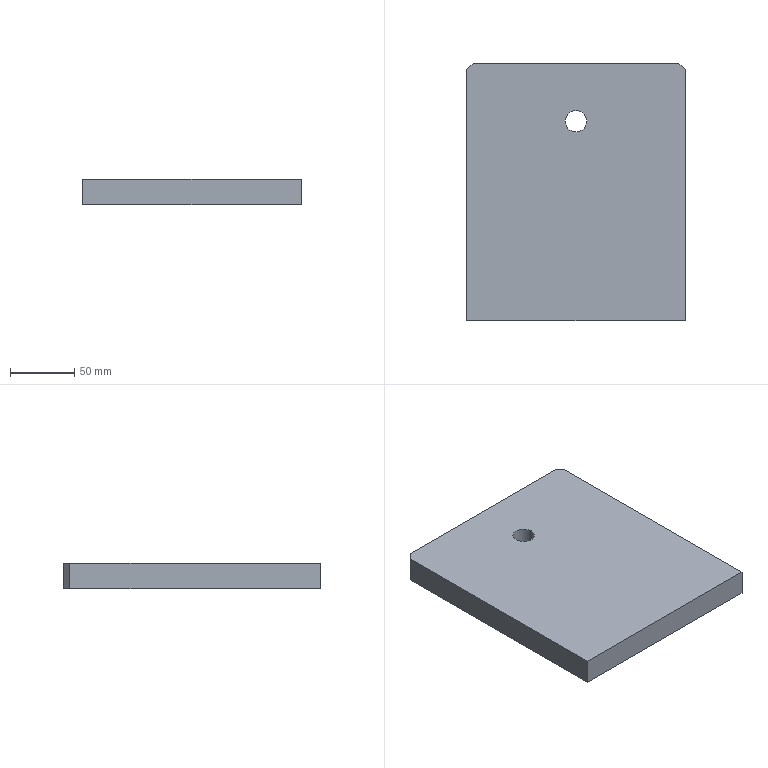Part | SolidWorks | features 3DProfileFeature 1, Extrusion 1, HoleWzd 1 | 1 solid | 10 faces | box 170 x 200 x 20 mm | volume 675136 mm3 | plane 8 | cylinder 2 | commonest cylinder face diameters 16.667 x2
STEP:
#1=CARTESIAN_POINT('',(76.666,155.,0.));
#2=VERTEX_POINT('',#1);
#3=CARTESIAN_POINT('',(93.334,155.,0.));
#4=VERTEX_POINT('',#3);
#5=CARTESIAN_POINT('',(85.,155.,0.));
#6=DIRECTION('',(0.,0.,1.));
#7=DIRECTION('',(1.,0.,0.));
#8=AXIS2_PLACEMENT_3D('',#5,#6,#7);
#9=CIRCLE('',#8,8.334);
#10=EDGE_CURVE('',#2,#4,#9,.T.);
#11=ORIENTED_EDGE('',*,*,#10,.F.);
#12=CARTESIAN_POINT('',(76.666,155.,20.));
#13=VERTEX_POINT('',#12);
#14=CARTESIAN_POINT('',(76.666,155.,20.));
#15=DIRECTION('',(0.,0.,1.));
#16=VECTOR('',#15,1000.);
#17=LINE('',#14,#16);
#18=EDGE_CURVE('',#2,#13,#17,.T.);
#19=ORIENTED_EDGE('',*,*,#18,.T.);
#20=CARTESIAN_POINT('',(93.334,155.,20.));
#21=VERTEX_POINT('',#20);
#22=CARTESIAN_POINT('',(85.,155.,20.));
#23=DIRECTION('',(0.,0.,1.));
#24=DIRECTION('',(1.,0.,0.));
#25=AXIS2_PLACEMENT_3D('',#22,#23,#24);
#26=CIRCLE('',#25,8.334);
#27=EDGE_CURVE('',#13,#21,#26,.T.);
#28=ORIENTED_EDGE('',*,*,#27,.T.);
#29=CARTESIAN_POINT('',(93.334,155.,20.));
#30=DIRECTION('',(0.,0.,1.));
#31=VECTOR('',#30,1000.);
#32=LINE('',#29,#31);
#33=EDGE_CURVE('',#4,#21,#32,.T.);
#34=ORIENTED_EDGE('',*,*,#33,.F.);
#35=EDGE_LOOP('',(#11,#19,#28,#34));
#36=FACE_OUTER_BOUND('',#35,.T.);
#37=CARTESIAN_POINT('',(85.,155.,20.));
#38=DIRECTION('',(0.,0.,1.));
#39=DIRECTION('',(1.,0.,0.));
#40=AXIS2_PLACEMENT_3D('',#37,#38,#39);
#41=CYLINDRICAL_SURFACE('',#40,8.334);
#42=ADVANCED_FACE('',(#36),#41,.F.);
#43=CARTESIAN_POINT('',(0.,195.,0.));
#44=VERTEX_POINT('',#43);
#45=CARTESIAN_POINT('',(0.,0.,0.));
#46=VERTEX_POINT('',#45);
#47=CARTESIAN_POINT('',(0.,0.,0.));
#48=DIRECTION('',(0.,-1.,0.));
#49=VECTOR('',#48,1000.);
#50=LINE('',#47,#49);
#51=EDGE_CURVE('',#44,#46,#50,.T.);
#52=ORIENTED_EDGE('',*,*,#51,.T.);
#53=CARTESIAN_POINT('',(0.,0.,20.));
#54=VERTEX_POINT('',#53);
#55=CARTESIAN_POINT('',(0.,0.,20.));
#56=DIRECTION('',(0.,0.,-1.));
#57=VECTOR('',#56,1000.);
#58=LINE('',#55,#57);
#59=EDGE_CURVE('',#54,#46,#58,.T.);
#60=ORIENTED_EDGE('',*,*,#59,.F.);
#61=CARTESIAN_POINT('',(0.,195.,20.));
#62=VERTEX_POINT('',#61);
#63=CARTESIAN_POINT('',(0.,0.,20.));
#64=DIRECTION('',(0.,-1.,0.));
#65=VECTOR('',#64,1000.);
#66=LINE('',#63,#65);
#67=EDGE_CURVE('',#62,#54,#66,.T.);
#68=ORIENTED_EDGE('',*,*,#67,.F.);
#69=CARTESIAN_POINT('',(0.,195.,20.));
#70=DIRECTION('',(0.,0.,-1.));
#71=VECTOR('',#70,1000.);
#72=LINE('',#69,#71);
#73=EDGE_CURVE('',#62,#44,#72,.T.);
#74=ORIENTED_EDGE('',*,*,#73,.T.);
#75=EDGE_LOOP('',(#52,#60,#68,#74));
#76=FACE_OUTER_BOUND('',#75,.T.);
#77=CARTESIAN_POINT('',(0.,0.,20.));
#78=DIRECTION('',(1.,0.,0.));
#79=DIRECTION('',(0.,0.,-1.));
#80=AXIS2_PLACEMENT_3D('',#77,#78,#79);
#81=PLANE('',#80);
#82=ADVANCED_FACE('',(#76),#81,.F.);
#83=CARTESIAN_POINT('',(170.,0.,0.));
#84=VERTEX_POINT('',#83);
#85=CARTESIAN_POINT('',(0.,0.,0.));
#86=DIRECTION('',(1.,0.,0.));
#87=VECTOR('',#86,1000.);
#88=LINE('',#85,#87);
#89=EDGE_CURVE('',#46,#84,#88,.T.);
#90=ORIENTED_EDGE('',*,*,#89,.T.);
#91=CARTESIAN_POINT('',(170.,0.,20.));
#92=VERTEX_POINT('',#91);
#93=CARTESIAN_POINT('',(170.,0.,20.));
#94=DIRECTION('',(0.,0.,-1.));
#95=VECTOR('',#94,1000.);
#96=LINE('',#93,#95);
#97=EDGE_CURVE('',#92,#84,#96,.T.);
#98=ORIENTED_EDGE('',*,*,#97,.F.);
#99=CARTESIAN_POINT('',(0.,0.,20.));
#100=DIRECTION('',(1.,0.,0.));
#101=VECTOR('',#100,1000.);
#102=LINE('',#99,#101);
#103=EDGE_CURVE('',#54,#92,#102,.T.);
#104=ORIENTED_EDGE('',*,*,#103,.F.);
#105=ORIENTED_EDGE('',*,*,#59,.T.);
#106=EDGE_LOOP('',(#90,#98,#104,#105));
#107=FACE_OUTER_BOUND('',#106,.T.);
#108=CARTESIAN_POINT('',(0.,0.,20.));
#109=DIRECTION('',(0.,1.,0.));
#110=DIRECTION('',(0.,0.,1.));
#111=AXIS2_PLACEMENT_3D('',#108,#109,#110);
#112=PLANE('',#111);
#113=ADVANCED_FACE('',(#107),#112,.F.);
#114=CARTESIAN_POINT('',(170.,195.,0.));
#115=VERTEX_POINT('',#114);
#116=CARTESIAN_POINT('',(170.,0.,0.));
#117=DIRECTION('',(0.,1.,0.));
#118=VECTOR('',#117,1000.);
#119=LINE('',#116,#118);
#120=EDGE_CURVE('',#84,#115,#119,.T.);
#121=ORIENTED_EDGE('',*,*,#120,.T.);
#122=CARTESIAN_POINT('',(170.,195.,20.));
#123=VERTEX_POINT('',#122);
#124=CARTESIAN_POINT('',(170.,195.,20.));
#125=DIRECTION('',(0.,0.,-1.));
#126=VECTOR('',#125,1000.);
#127=LINE('',#124,#126);
#128=EDGE_CURVE('',#123,#115,#127,.T.);
#129=ORIENTED_EDGE('',*,*,#128,.F.);
#130=CARTESIAN_POINT('',(170.,0.,20.));
#131=DIRECTION('',(0.,1.,0.));
#132=VECTOR('',#131,1000.);
#133=LINE('',#130,#132);
#134=EDGE_CURVE('',#92,#123,#133,.T.);
#135=ORIENTED_EDGE('',*,*,#134,.F.);
#136=ORIENTED_EDGE('',*,*,#97,.T.);
#137=EDGE_LOOP('',(#121,#129,#135,#136));
#138=FACE_OUTER_BOUND('',#137,.T.);
#139=CARTESIAN_POINT('',(170.,0.,20.));
#140=DIRECTION('',(-1.,0.,0.));
#141=DIRECTION('',(0.,0.,1.));
#142=AXIS2_PLACEMENT_3D('',#139,#140,#141);
#143=PLANE('',#142);
#144=ADVANCED_FACE('',(#138),#143,.F.);
#145=CARTESIAN_POINT('',(165.,200.,0.));
#146=VERTEX_POINT('',#145);
#147=CARTESIAN_POINT('',(165.,200.,0.));
#148=DIRECTION('',(-0.7071,0.7071,0.));
#149=VECTOR('',#148,1000.);
#150=LINE('',#147,#149);
#151=EDGE_CURVE('',#115,#146,#150,.T.);
#152=ORIENTED_EDGE('',*,*,#151,.T.);
#153=CARTESIAN_POINT('',(165.,200.,20.));
#154=VERTEX_POINT('',#153);
#155=CARTESIAN_POINT('',(165.,200.,20.));
#156=DIRECTION('',(0.,0.,-1.));
#157=VECTOR('',#156,1000.);
#158=LINE('',#155,#157);
#159=EDGE_CURVE('',#154,#146,#158,.T.);
#160=ORIENTED_EDGE('',*,*,#159,.F.);
#161=CARTESIAN_POINT('',(165.,200.,20.));
#162=DIRECTION('',(-0.7071,0.7071,0.));
#163=VECTOR('',#162,1000.);
#164=LINE('',#161,#163);
#165=EDGE_CURVE('',#123,#154,#164,.T.);
#166=ORIENTED_EDGE('',*,*,#165,.F.);
#167=ORIENTED_EDGE('',*,*,#128,.T.);
#168=EDGE_LOOP('',(#152,#160,#166,#167));
#169=FACE_OUTER_BOUND('',#168,.T.);
#170=CARTESIAN_POINT('',(165.,200.,20.));
#171=DIRECTION('',(-0.7071,-0.7071,0.));
#172=DIRECTION('',(0.7071,-0.7071,0.));
#173=AXIS2_PLACEMENT_3D('',#170,#171,#172);
#174=PLANE('',#173);
#175=ADVANCED_FACE('',(#169),#174,.F.);
#176=CARTESIAN_POINT('',(5.,200.,0.));
#177=VERTEX_POINT('',#176);
#178=CARTESIAN_POINT('',(5.,200.,0.));
#179=DIRECTION('',(-1.,0.,0.));
#180=VECTOR('',#179,1000.);
#181=LINE('',#178,#180);
#182=EDGE_CURVE('',#146,#177,#181,.T.);
#183=ORIENTED_EDGE('',*,*,#182,.T.);
#184=CARTESIAN_POINT('',(5.,200.,20.));
#185=VERTEX_POINT('',#184);
#186=CARTESIAN_POINT('',(5.,200.,20.));
#187=DIRECTION('',(0.,0.,-1.));
#188=VECTOR('',#187,1000.);
#189=LINE('',#186,#188);
#190=EDGE_CURVE('',#185,#177,#189,.T.);
#191=ORIENTED_EDGE('',*,*,#190,.F.);
#192=CARTESIAN_POINT('',(5.,200.,20.));
#193=DIRECTION('',(-1.,0.,0.));
#194=VECTOR('',#193,1000.);
#195=LINE('',#192,#194);
#196=EDGE_CURVE('',#154,#185,#195,.T.);
#197=ORIENTED_EDGE('',*,*,#196,.F.);
#198=ORIENTED_EDGE('',*,*,#159,.T.);
#199=EDGE_LOOP('',(#183,#191,#197,#198));
#200=FACE_OUTER_BOUND('',#199,.T.);
#201=CARTESIAN_POINT('',(5.,200.,20.));
#202=DIRECTION('',(0.,-1.,0.));
#203=DIRECTION('',(0.,0.,-1.));
#204=AXIS2_PLACEMENT_3D('',#201,#202,#203);
#205=PLANE('',#204);
#206=ADVANCED_FACE('',(#200),#205,.F.);
#207=CARTESIAN_POINT('',(0.,195.,0.));
#208=DIRECTION('',(-0.7071,-0.7071,0.));
#209=VECTOR('',#208,1000.);
#210=LINE('',#207,#209);
#211=EDGE_CURVE('',#177,#44,#210,.T.);
#212=ORIENTED_EDGE('',*,*,#211,.T.);
#213=ORIENTED_EDGE('',*,*,#73,.F.);
#214=CARTESIAN_POINT('',(0.,195.,20.));
#215=DIRECTION('',(-0.7071,-0.7071,0.));
#216=VECTOR('',#215,1000.);
#217=LINE('',#214,#216);
#218=EDGE_CURVE('',#185,#62,#217,.T.);
#219=ORIENTED_EDGE('',*,*,#218,.F.);
#220=ORIENTED_EDGE('',*,*,#190,.T.);
#221=EDGE_LOOP('',(#212,#213,#219,#220));
#222=FACE_OUTER_BOUND('',#221,.T.);
#223=CARTESIAN_POINT('',(0.,195.,20.));
#224=DIRECTION('',(0.7071,-0.7071,0.));
#225=DIRECTION('',(0.7071,0.7071,0.));
#226=AXIS2_PLACEMENT_3D('',#223,#224,#225);
#227=PLANE('',#226);
#228=ADVANCED_FACE('',(#222),#227,.F.);
#229=CARTESIAN_POINT('',(85.,155.,20.));
#230=DIRECTION('',(0.,0.,1.));
#231=DIRECTION('',(1.,0.,0.));
#232=AXIS2_PLACEMENT_3D('',#229,#230,#231);
#233=CIRCLE('',#232,8.334);
#234=EDGE_CURVE('',#21,#13,#233,.T.);
#235=ORIENTED_EDGE('',*,*,#234,.F.);
#236=ORIENTED_EDGE('',*,*,#27,.F.);
#237=EDGE_LOOP('',(#235,#236));
#238=FACE_BOUND('',#237,.T.);
#239=ORIENTED_EDGE('',*,*,#67,.T.);
#240=ORIENTED_EDGE('',*,*,#103,.T.);
#241=ORIENTED_EDGE('',*,*,#134,.T.);
#242=ORIENTED_EDGE('',*,*,#165,.T.);
#243=ORIENTED_EDGE('',*,*,#196,.T.);
#244=ORIENTED_EDGE('',*,*,#218,.T.);
#245=EDGE_LOOP('',(#239,#240,#241,#242,#243,#244));
#246=FACE_OUTER_BOUND('',#245,.T.);
#247=CARTESIAN_POINT('',(0.,0.,20.));
#248=DIRECTION('',(0.,0.,-1.));
#249=DIRECTION('',(-1.,0.,0.));
#250=AXIS2_PLACEMENT_3D('',#247,#248,#249);
#251=PLANE('',#250);
#252=ADVANCED_FACE('',(#238,#246),#251,.F.);
#253=CARTESIAN_POINT('',(85.,155.,0.));
#254=DIRECTION('',(0.,0.,1.));
#255=DIRECTION('',(1.,0.,0.));
#256=AXIS2_PLACEMENT_3D('',#253,#254,#255);
#257=CIRCLE('',#256,8.334);
#258=EDGE_CURVE('',#4,#2,#257,.T.);
#259=ORIENTED_EDGE('',*,*,#258,.T.);
#260=ORIENTED_EDGE('',*,*,#10,.T.);
#261=EDGE_LOOP('',(#259,#260));
#262=FACE_BOUND('',#261,.T.);
#263=ORIENTED_EDGE('',*,*,#51,.F.);
#264=ORIENTED_EDGE('',*,*,#211,.F.);
#265=ORIENTED_EDGE('',*,*,#182,.F.);
#266=ORIENTED_EDGE('',*,*,#151,.F.);
#267=ORIENTED_EDGE('',*,*,#120,.F.);
#268=ORIENTED_EDGE('',*,*,#89,.F.);
#269=EDGE_LOOP('',(#263,#264,#265,#266,#267,#268));
#270=FACE_OUTER_BOUND('',#269,.T.);
#271=CARTESIAN_POINT('',(0.,0.,0.));
#272=DIRECTION('',(0.,0.,-1.));
#273=DIRECTION('',(-1.,0.,0.));
#274=AXIS2_PLACEMENT_3D('',#271,#272,#273);
#275=PLANE('',#274);
#276=ADVANCED_FACE('',(#262,#270),#275,.T.);
#277=ORIENTED_EDGE('',*,*,#18,.F.);
#278=ORIENTED_EDGE('',*,*,#258,.F.);
#279=ORIENTED_EDGE('',*,*,#33,.T.);
#280=ORIENTED_EDGE('',*,*,#234,.T.);
#281=EDGE_LOOP('',(#277,#278,#279,#280));
#282=FACE_OUTER_BOUND('',#281,.T.);
#283=CARTESIAN_POINT('',(85.,155.,20.));
#284=DIRECTION('',(0.,0.,1.));
#285=DIRECTION('',(1.,0.,0.));
#286=AXIS2_PLACEMENT_3D('',#283,#284,#285);
#287=CYLINDRICAL_SURFACE('',#286,8.334);
#288=ADVANCED_FACE('',(#282),#287,.F.);
#289=CLOSED_SHELL('',(#42,#82,#113,#144,#175,#206,#228,#252,#276,#288));
#290=MANIFOLD_SOLID_BREP('',#289);
#291=CARTESIAN_POINT('',(0.,0.,0.));
#292=DIRECTION('',(0.,0.,1.));
#293=DIRECTION('',(1.,0.,0.));
#294=AXIS2_PLACEMENT_3D('',#291,#292,#293);
#295=(LENGTH_UNIT()NAMED_UNIT(*)SI_UNIT(.MILLI.,.METRE.));
#296=UNCERTAINTY_MEASURE_WITH_UNIT(LENGTH_MEASURE(0.00001),#295,'','');
#297=(NAMED_UNIT(*)PLANE_ANGLE_UNIT()SI_UNIT($,.RADIAN.));
#298=(NAMED_UNIT(*)SI_UNIT($,.STERADIAN.)SOLID_ANGLE_UNIT());
#299=(GEOMETRIC_REPRESENTATION_CONTEXT(3)GLOBAL_UNCERTAINTY_ASSIGNED_CONTEXT((#296))GLOBAL_UNIT_ASSIGNED_CONTEXT((#295,#297,#298))REPRESENTATION_CONTEXT('',''));
#300=ADVANCED_BREP_SHAPE_REPRESENTATION('',(#290,#294),#299);